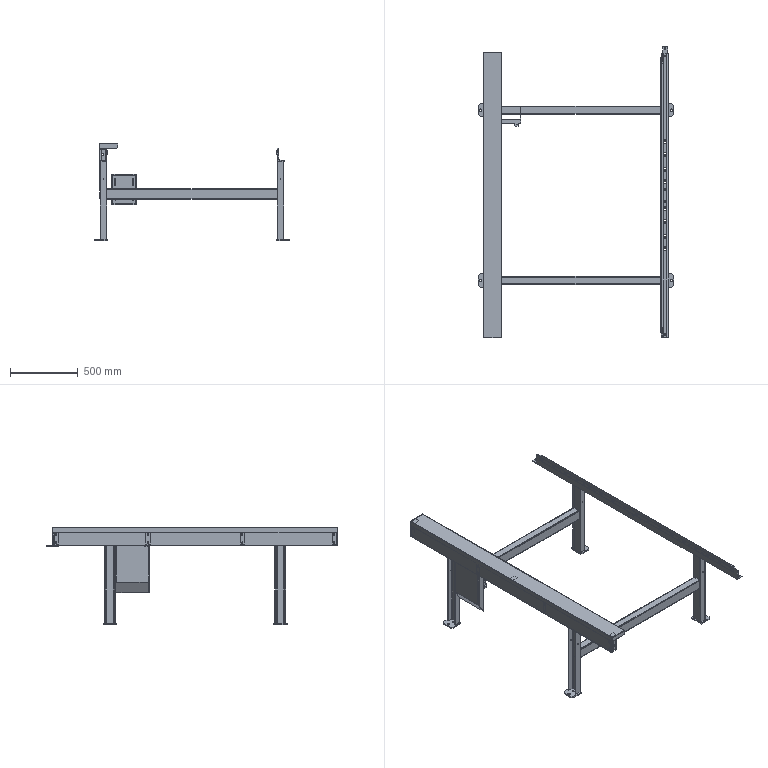Part | SolidWorks | 35 solids | 956 faces | box 1444 x 2158 x 720 mm | volume 13772315 mm3 | plane 524 | cylinder 427 | spline 5 | commonest cylinder face diameters 13 x76 6 x68 10.5 x52 5 x40 20 x38 11 x36